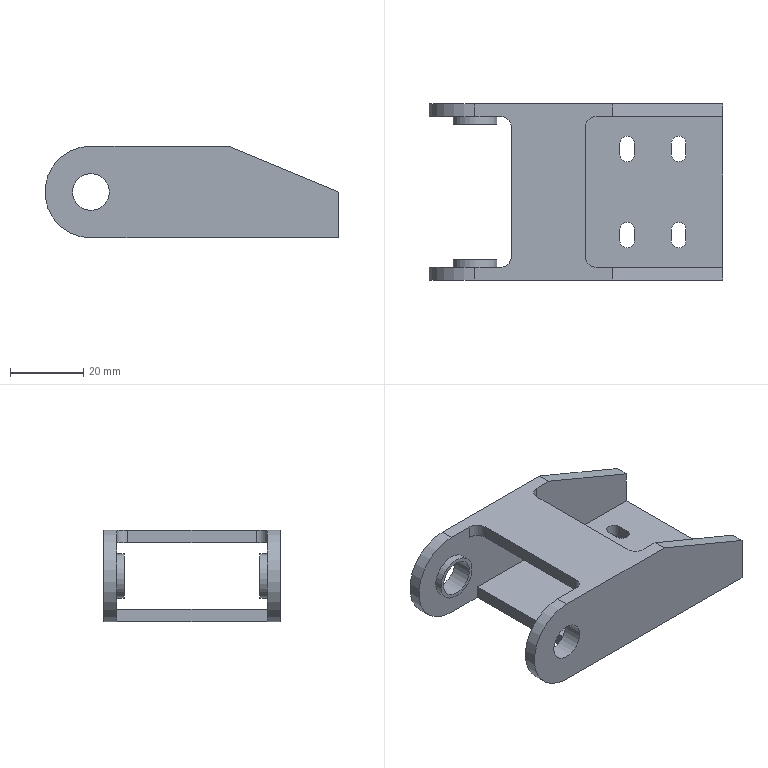Part | STEP file | 1 solid | 42 faces | box 80 x 48 x 25 mm | volume 22611 mm3 | plane 24 | cylinder 18 | commonest cylinder face diameters 4 x8 6 x4 10 x2 12 x2 25 x2